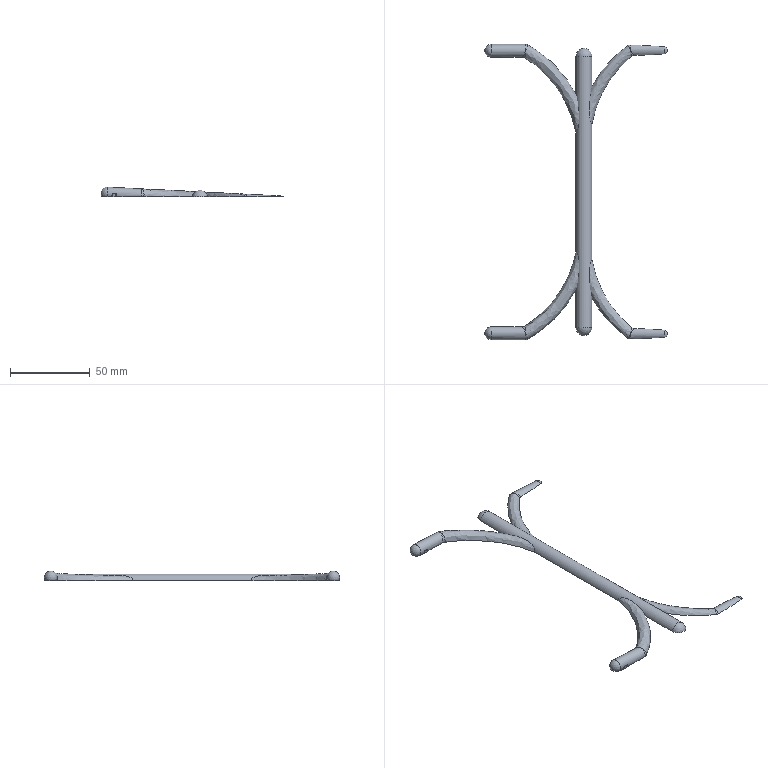Part | STEP file | solid 214 | 1 solid | 40 faces | box 114.278 x 185.224 x 7.51 mm | volume 11384 mm3 | spline 24 | sphere 6 | plane 5 | cylinder 5 | commonest cylinder face diameters 8 x4 10 x1